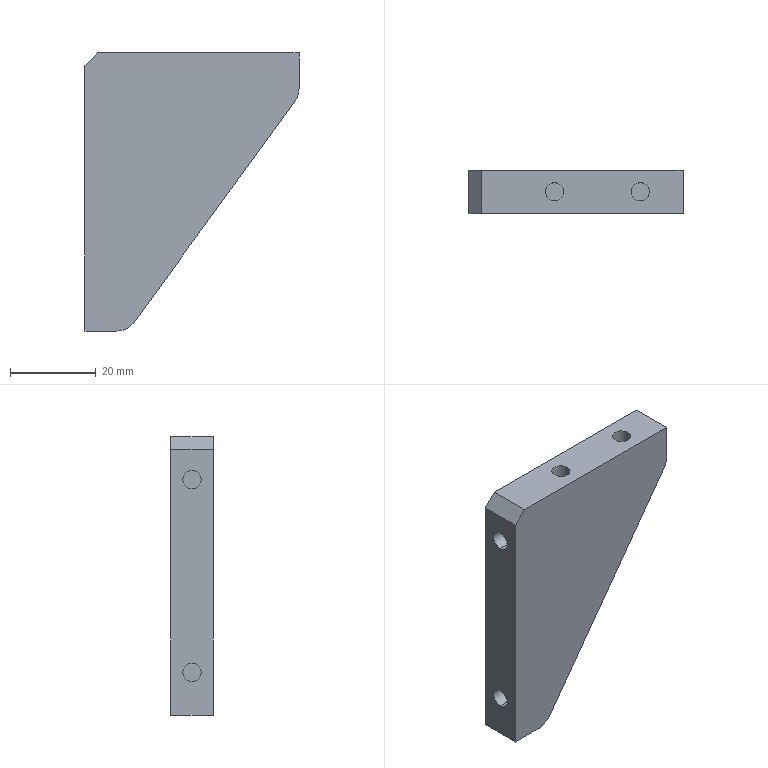Part | STEP file | PN_0009 | 1 solid | 22 faces | box 50 x 10 x 65 mm | volume 20426 mm3 | plane 12 | cylinder 10 | commonest cylinder face diameters 4.3 x8 10 x2
STEP:
#1=CARTESIAN_POINT('',(0.,0.,0.));
#2=DIRECTION('',(0.,0.,1.));
#3=DIRECTION('',(1.,0.,0.));
#4=AXIS2_PLACEMENT_3D('',#1,#2,#3);
#5=CARTESIAN_POINT('',(142.2,-67.,62.));
#6=VERTEX_POINT('',#5);
#7=CARTESIAN_POINT('',(139.2,-67.,59.));
#8=VERTEX_POINT('',#7);
#9=CARTESIAN_POINT('',(142.2,-67.,62.));
#10=DIRECTION('',(-0.7071,0.,-0.7071));
#11=VECTOR('',#10,1.);
#12=LINE('',#9,#11);
#13=CARTESIAN_POINT('',(0.,-67.,0.));
#14=DIRECTION('',(0.,-1.,0.));
#15=DIRECTION('',(1.,0.,0.));
#16=AXIS2_PLACEMENT_3D('',#13,#14,#15);
#17=PLANE('',#16);
#18=CARTESIAN_POINT('',(142.2,62.));
#19=DIRECTION('',(-0.7071,-0.7071));
#20=VECTOR('',#19,1.);
#21=LINE('',#18,#20);
#22=(GEOMETRIC_REPRESENTATION_CONTEXT(2)PARAMETRIC_REPRESENTATION_CONTEXT()REPRESENTATION_CONTEXT('',''));
#23=DEFINITIONAL_REPRESENTATION('',(#21),#22);
#24=PCURVE('',#17,#23);
#25=CARTESIAN_POINT('',(140.7,-62.,60.5));
#26=DIRECTION('',(-0.7071,0.,0.7071));
#27=DIRECTION('',(0.7071,0.,0.7071));
#28=AXIS2_PLACEMENT_3D('',#25,#26,#27);
#29=PLANE('',#28);
#30=CARTESIAN_POINT('',(2.121,-5.));
#31=DIRECTION('',(-1.,0.));
#32=VECTOR('',#31,1.);
#33=LINE('',#30,#32);
#34=(GEOMETRIC_REPRESENTATION_CONTEXT(2)PARAMETRIC_REPRESENTATION_CONTEXT()REPRESENTATION_CONTEXT('',''));
#35=DEFINITIONAL_REPRESENTATION('',(#33),#34);
#36=PCURVE('',#29,#35);
#37=SURFACE_CURVE('',#12,(#24,#36),.PCURVE_S1.);
#38=EDGE_CURVE('',#6,#8,#37,.T.);
#39=ORIENTED_EDGE('',*,*,#38,.F.);
#40=CARTESIAN_POINT('',(189.2,-67.,62.));
#41=VERTEX_POINT('',#40);
#42=CARTESIAN_POINT('',(189.2,-67.,62.));
#43=DIRECTION('',(-1.,0.,0.));
#44=VECTOR('',#43,1.);
#45=LINE('',#42,#44);
#46=CARTESIAN_POINT('',(189.2,62.));
#47=DIRECTION('',(-1.,0.));
#48=VECTOR('',#47,1.);
#49=LINE('',#46,#48);
#50=(GEOMETRIC_REPRESENTATION_CONTEXT(2)PARAMETRIC_REPRESENTATION_CONTEXT()REPRESENTATION_CONTEXT('',''));
#51=DEFINITIONAL_REPRESENTATION('',(#49),#50);
#52=PCURVE('',#17,#51);
#53=CARTESIAN_POINT('',(189.2,-67.,62.));
#54=DIRECTION('',(0.,0.,1.));
#55=DIRECTION('',(-1.,0.,0.));
#56=AXIS2_PLACEMENT_3D('',#53,#54,#55);
#57=PLANE('',#56);
#58=CARTESIAN_POINT('',(0.,0.));
#59=DIRECTION('',(1.,0.));
#60=VECTOR('',#59,1.);
#61=LINE('',#58,#60);
#62=(GEOMETRIC_REPRESENTATION_CONTEXT(2)PARAMETRIC_REPRESENTATION_CONTEXT()REPRESENTATION_CONTEXT('',''));
#63=DEFINITIONAL_REPRESENTATION('',(#61),#62);
#64=PCURVE('',#57,#63);
#65=SURFACE_CURVE('',#45,(#52,#64),.PCURVE_S1.);
#66=EDGE_CURVE('',#41,#6,#65,.T.);
#67=ORIENTED_EDGE('',*,*,#66,.F.);
#68=CARTESIAN_POINT('',(189.2,-67.,53.626));
#69=VERTEX_POINT('',#68);
#70=CARTESIAN_POINT('',(189.2,-67.,53.626));
#71=DIRECTION('',(0.,0.,1.));
#72=VECTOR('',#71,1.);
#73=LINE('',#70,#72);
#74=CARTESIAN_POINT('',(189.2,53.626));
#75=DIRECTION('',(0.,1.));
#76=VECTOR('',#75,1.);
#77=LINE('',#74,#76);
#78=(GEOMETRIC_REPRESENTATION_CONTEXT(2)PARAMETRIC_REPRESENTATION_CONTEXT()REPRESENTATION_CONTEXT('',''));
#79=DEFINITIONAL_REPRESENTATION('',(#77),#78);
#80=PCURVE('',#17,#79);
#81=CARTESIAN_POINT('',(189.2,-67.,52.));
#82=DIRECTION('',(1.,0.,0.));
#83=DIRECTION('',(0.,0.,1.));
#84=AXIS2_PLACEMENT_3D('',#81,#82,#83);
#85=PLANE('',#84);
#86=CARTESIAN_POINT('',(1.626,0.));
#87=DIRECTION('',(1.,0.));
#88=VECTOR('',#87,1.);
#89=LINE('',#86,#88);
#90=(GEOMETRIC_REPRESENTATION_CONTEXT(2)PARAMETRIC_REPRESENTATION_CONTEXT()REPRESENTATION_CONTEXT('',''));
#91=DEFINITIONAL_REPRESENTATION('',(#89),#90);
#92=PCURVE('',#85,#91);
#93=SURFACE_CURVE('',#73,(#80,#92),.PCURVE_S1.);
#94=EDGE_CURVE('',#69,#41,#93,.T.);
#95=ORIENTED_EDGE('',*,*,#94,.F.);
#96=CARTESIAN_POINT('',(188.244,-67.,50.685));
#97=VERTEX_POINT('',#96);
#98=CARTESIAN_POINT('',(184.2,-67.,53.626));
#99=DIRECTION('',(0.,-1.,0.));
#100=DIRECTION('',(0.8087,0.,-0.5882));
#101=AXIS2_PLACEMENT_3D('',#98,#99,#100);
#102=CIRCLE('',#101,5.);
#103=CARTESIAN_POINT('',(184.2,53.626));
#104=DIRECTION('',(0.8087,-0.5882));
#105=AXIS2_PLACEMENT_2D('',#103,#104);
#106=CIRCLE('',#105,5.);
#107=(GEOMETRIC_REPRESENTATION_CONTEXT(2)PARAMETRIC_REPRESENTATION_CONTEXT()REPRESENTATION_CONTEXT('',''));
#108=DEFINITIONAL_REPRESENTATION('',(#106),#107);
#109=PCURVE('',#17,#108);
#110=CARTESIAN_POINT('',(184.2,-67.129,53.626));
#111=DIRECTION('',(0.,1.,0.));
#112=DIRECTION('',(1.,0.,0.));
#113=AXIS2_PLACEMENT_3D('',#110,#111,#112);
#114=CYLINDRICAL_SURFACE('',#113,5.);
#115=CARTESIAN_POINT('',(0.6288,0.1293));
#116=DIRECTION('',(-1.,0.));
#117=VECTOR('',#116,1.);
#118=LINE('',#115,#117);
#119=(GEOMETRIC_REPRESENTATION_CONTEXT(2)PARAMETRIC_REPRESENTATION_CONTEXT()REPRESENTATION_CONTEXT('',''));
#120=DEFINITIONAL_REPRESENTATION('',(#118),#119);
#121=PCURVE('',#114,#120);
#122=SURFACE_CURVE('',#102,(#109,#121),.PCURVE_S1.);
#123=EDGE_CURVE('',#97,#69,#122,.T.);
#124=ORIENTED_EDGE('',*,*,#123,.F.);
#125=CARTESIAN_POINT('',(150.698,-67.,-0.9409));
#126=VERTEX_POINT('',#125);
#127=CARTESIAN_POINT('',(150.698,-67.,-0.9409));
#128=DIRECTION('',(0.5882,0.,0.8087));
#129=VECTOR('',#128,1.);
#130=LINE('',#127,#129);
#131=CARTESIAN_POINT('',(150.698,-0.9409));
#132=DIRECTION('',(0.5882,0.8087));
#133=VECTOR('',#132,1.);
#134=LINE('',#131,#133);
#135=(GEOMETRIC_REPRESENTATION_CONTEXT(2)PARAMETRIC_REPRESENTATION_CONTEXT()REPRESENTATION_CONTEXT('',''));
#136=DEFINITIONAL_REPRESENTATION('',(#134),#135);
#137=PCURVE('',#17,#136);
#138=CARTESIAN_POINT('',(149.2,-67.,-3.));
#139=DIRECTION('',(0.8087,0.,-0.5882));
#140=DIRECTION('',(0.5882,0.,0.8087));
#141=AXIS2_PLACEMENT_3D('',#138,#139,#140);
#142=PLANE('',#141);
#143=CARTESIAN_POINT('',(2.546,0.));
#144=DIRECTION('',(1.,0.));
#145=VECTOR('',#144,1.);
#146=LINE('',#143,#145);
#147=(GEOMETRIC_REPRESENTATION_CONTEXT(2)PARAMETRIC_REPRESENTATION_CONTEXT()REPRESENTATION_CONTEXT('',''));
#148=DEFINITIONAL_REPRESENTATION('',(#146),#147);
#149=PCURVE('',#142,#148);
#150=SURFACE_CURVE('',#130,(#137,#149),.PCURVE_S1.);
#151=EDGE_CURVE('',#126,#97,#150,.T.);
#152=ORIENTED_EDGE('',*,*,#151,.F.);
#153=CARTESIAN_POINT('',(146.654,-67.,-3.));
#154=VERTEX_POINT('',#153);
#155=CARTESIAN_POINT('',(146.654,-67.,2.));
#156=DIRECTION('',(0.,-1.,0.));
#157=DIRECTION('',(0.,0.,-1.));
#158=AXIS2_PLACEMENT_3D('',#155,#156,#157);
#159=CIRCLE('',#158,5.);
#160=CARTESIAN_POINT('',(146.654,2.));
#161=DIRECTION('',(0.,-1.));
#162=AXIS2_PLACEMENT_2D('',#160,#161);
#163=CIRCLE('',#162,5.);
#164=(GEOMETRIC_REPRESENTATION_CONTEXT(2)PARAMETRIC_REPRESENTATION_CONTEXT()REPRESENTATION_CONTEXT('',''));
#165=DEFINITIONAL_REPRESENTATION('',(#163),#164);
#166=PCURVE('',#17,#165);
#167=CARTESIAN_POINT('',(146.654,-67.129,2.));
#168=DIRECTION('',(0.,1.,0.));
#169=DIRECTION('',(0.8087,0.,-0.5882));
#170=AXIS2_PLACEMENT_3D('',#167,#168,#169);
#171=CYLINDRICAL_SURFACE('',#170,5.);
#172=CARTESIAN_POINT('',(0.942,0.1293));
#173=DIRECTION('',(-1.,0.));
#174=VECTOR('',#173,1.);
#175=LINE('',#172,#174);
#176=(GEOMETRIC_REPRESENTATION_CONTEXT(2)PARAMETRIC_REPRESENTATION_CONTEXT()REPRESENTATION_CONTEXT('',''));
#177=DEFINITIONAL_REPRESENTATION('',(#175),#176);
#178=PCURVE('',#171,#177);
#179=SURFACE_CURVE('',#159,(#166,#178),.PCURVE_S1.);
#180=EDGE_CURVE('',#154,#126,#179,.T.);
#181=ORIENTED_EDGE('',*,*,#180,.F.);
#182=CARTESIAN_POINT('',(139.2,-67.,-3.));
#183=VERTEX_POINT('',#182);
#184=CARTESIAN_POINT('',(139.2,-67.,-3.));
#185=DIRECTION('',(1.,0.,0.));
#186=VECTOR('',#185,1.);
#187=LINE('',#184,#186);
#188=CARTESIAN_POINT('',(139.2,-3.));
#189=DIRECTION('',(1.,0.));
#190=VECTOR('',#189,1.);
#191=LINE('',#188,#190);
#192=(GEOMETRIC_REPRESENTATION_CONTEXT(2)PARAMETRIC_REPRESENTATION_CONTEXT()REPRESENTATION_CONTEXT('',''));
#193=DEFINITIONAL_REPRESENTATION('',(#191),#192);
#194=PCURVE('',#17,#193);
#195=CARTESIAN_POINT('',(139.2,-67.,-3.));
#196=DIRECTION('',(0.,0.,-1.));
#197=DIRECTION('',(1.,0.,0.));
#198=AXIS2_PLACEMENT_3D('',#195,#196,#197);
#199=PLANE('',#198);
#200=CARTESIAN_POINT('',(0.,0.));
#201=DIRECTION('',(1.,0.));
#202=VECTOR('',#201,1.);
#203=LINE('',#200,#202);
#204=(GEOMETRIC_REPRESENTATION_CONTEXT(2)PARAMETRIC_REPRESENTATION_CONTEXT()REPRESENTATION_CONTEXT('',''));
#205=DEFINITIONAL_REPRESENTATION('',(#203),#204);
#206=PCURVE('',#199,#205);
#207=SURFACE_CURVE('',#187,(#194,#206),.PCURVE_S1.);
#208=EDGE_CURVE('',#183,#154,#207,.T.);
#209=ORIENTED_EDGE('',*,*,#208,.F.);
#210=CARTESIAN_POINT('',(139.2,-67.,59.));
#211=DIRECTION('',(0.,0.,-1.));
#212=VECTOR('',#211,1.);
#213=LINE('',#210,#212);
#214=CARTESIAN_POINT('',(139.2,59.));
#215=DIRECTION('',(0.,-1.));
#216=VECTOR('',#215,1.);
#217=LINE('',#214,#216);
#218=(GEOMETRIC_REPRESENTATION_CONTEXT(2)PARAMETRIC_REPRESENTATION_CONTEXT()REPRESENTATION_CONTEXT('',''));
#219=DEFINITIONAL_REPRESENTATION('',(#217),#218);
#220=PCURVE('',#17,#219);
#221=CARTESIAN_POINT('',(139.2,-67.,62.));
#222=DIRECTION('',(-1.,0.,0.));
#223=DIRECTION('',(0.,0.,-1.));
#224=AXIS2_PLACEMENT_3D('',#221,#222,#223);
#225=PLANE('',#224);
#226=CARTESIAN_POINT('',(3.,0.));
#227=DIRECTION('',(1.,0.));
#228=VECTOR('',#227,1.);
#229=LINE('',#226,#228);
#230=(GEOMETRIC_REPRESENTATION_CONTEXT(2)PARAMETRIC_REPRESENTATION_CONTEXT()REPRESENTATION_CONTEXT('',''));
#231=DEFINITIONAL_REPRESENTATION('',(#229),#230);
#232=PCURVE('',#225,#231);
#233=SURFACE_CURVE('',#213,(#220,#232),.PCURVE_S1.);
#234=EDGE_CURVE('',#8,#183,#233,.T.);
#235=ORIENTED_EDGE('',*,*,#234,.F.);
#236=EDGE_LOOP('',(#39,#67,#95,#124,#152,#181,#209,#235));
#237=FACE_BOUND('',#236,.F.);
#238=ADVANCED_FACE('',(#237),#17,.T.);
#239=CARTESIAN_POINT('',(139.2,-57.,59.));
#240=VERTEX_POINT('',#239);
#241=CARTESIAN_POINT('',(142.2,-57.,62.));
#242=VERTEX_POINT('',#241);
#243=CARTESIAN_POINT('',(139.2,-57.,59.));
#244=DIRECTION('',(0.7071,0.,0.7071));
#245=VECTOR('',#244,1.);
#246=LINE('',#243,#245);
#247=CARTESIAN_POINT('',(-2.121,5.));
#248=DIRECTION('',(1.,0.));
#249=VECTOR('',#248,1.);
#250=LINE('',#247,#249);
#251=(GEOMETRIC_REPRESENTATION_CONTEXT(2)PARAMETRIC_REPRESENTATION_CONTEXT()REPRESENTATION_CONTEXT('',''));
#252=DEFINITIONAL_REPRESENTATION('',(#250),#251);
#253=PCURVE('',#29,#252);
#254=CARTESIAN_POINT('',(0.,-57.,0.));
#255=DIRECTION('',(0.,-1.,0.));
#256=DIRECTION('',(1.,0.,0.));
#257=AXIS2_PLACEMENT_3D('',#254,#255,#256);
#258=PLANE('',#257);
#259=CARTESIAN_POINT('',(139.2,59.));
#260=DIRECTION('',(0.7071,0.7071));
#261=VECTOR('',#260,1.);
#262=LINE('',#259,#261);
#263=(GEOMETRIC_REPRESENTATION_CONTEXT(2)PARAMETRIC_REPRESENTATION_CONTEXT()REPRESENTATION_CONTEXT('',''));
#264=DEFINITIONAL_REPRESENTATION('',(#262),#263);
#265=PCURVE('',#258,#264);
#266=SURFACE_CURVE('',#246,(#253,#265),.PCURVE_S1.);
#267=EDGE_CURVE('',#240,#242,#266,.T.);
#268=ORIENTED_EDGE('',*,*,#267,.T.);
#269=CARTESIAN_POINT('',(142.2,-67.,62.));
#270=DIRECTION('',(0.,1.,0.));
#271=VECTOR('',#270,1.);
#272=LINE('',#269,#271);
#273=CARTESIAN_POINT('',(2.121,-5.));
#274=DIRECTION('',(0.,1.));
#275=VECTOR('',#274,1.);
#276=LINE('',#273,#275);
#277=(GEOMETRIC_REPRESENTATION_CONTEXT(2)PARAMETRIC_REPRESENTATION_CONTEXT()REPRESENTATION_CONTEXT('',''));
#278=DEFINITIONAL_REPRESENTATION('',(#276),#277);
#279=PCURVE('',#29,#278);
#280=CARTESIAN_POINT('',(47.,0.));
#281=DIRECTION('',(0.,-1.));
#282=VECTOR('',#281,1.);
#283=LINE('',#280,#282);
#284=(GEOMETRIC_REPRESENTATION_CONTEXT(2)PARAMETRIC_REPRESENTATION_CONTEXT()REPRESENTATION_CONTEXT('',''));
#285=DEFINITIONAL_REPRESENTATION('',(#283),#284);
#286=PCURVE('',#57,#285);
#287=SURFACE_CURVE('',#272,(#279,#286),.PCURVE_S1.);
#288=EDGE_CURVE('',#6,#242,#287,.T.);
#289=ORIENTED_EDGE('',*,*,#288,.F.);
#290=ORIENTED_EDGE('',*,*,#38,.T.);
#291=CARTESIAN_POINT('',(139.2,-67.,59.));
#292=DIRECTION('',(0.,1.,0.));
#293=VECTOR('',#292,1.);
#294=LINE('',#291,#293);
#295=CARTESIAN_POINT('',(-2.121,-5.));
#296=DIRECTION('',(0.,1.));
#297=VECTOR('',#296,1.);
#298=LINE('',#295,#297);
#299=(GEOMETRIC_REPRESENTATION_CONTEXT(2)PARAMETRIC_REPRESENTATION_CONTEXT()REPRESENTATION_CONTEXT('',''));
#300=DEFINITIONAL_REPRESENTATION('',(#298),#299);
#301=PCURVE('',#29,#300);
#302=CARTESIAN_POINT('',(3.,0.));
#303=DIRECTION('',(0.,-1.));
#304=VECTOR('',#303,1.);
#305=LINE('',#302,#304);
#306=(GEOMETRIC_REPRESENTATION_CONTEXT(2)PARAMETRIC_REPRESENTATION_CONTEXT()REPRESENTATION_CONTEXT('',''));
#307=DEFINITIONAL_REPRESENTATION('',(#305),#306);
#308=PCURVE('',#225,#307);
#309=SURFACE_CURVE('',#294,(#301,#308),.PCURVE_S1.);
#310=EDGE_CURVE('',#8,#240,#309,.T.);
#311=ORIENTED_EDGE('',*,*,#310,.T.);
#312=EDGE_LOOP('',(#268,#289,#290,#311));
#313=FACE_BOUND('',#312,.F.);
#314=ADVANCED_FACE('',(#313),#29,.T.);
#315=ORIENTED_EDGE('',*,*,#267,.F.);
#316=CARTESIAN_POINT('',(139.2,-57.,-3.));
#317=VERTEX_POINT('',#316);
#318=CARTESIAN_POINT('',(139.2,-57.,59.));
#319=DIRECTION('',(0.,0.,-1.));
#320=VECTOR('',#319,1.);
#321=LINE('',#318,#320);
#322=CARTESIAN_POINT('',(139.2,59.));
#323=DIRECTION('',(0.,-1.));
#324=VECTOR('',#323,1.);
#325=LINE('',#322,#324);
#326=(GEOMETRIC_REPRESENTATION_CONTEXT(2)PARAMETRIC_REPRESENTATION_CONTEXT()REPRESENTATION_CONTEXT('',''));
#327=DEFINITIONAL_REPRESENTATION('',(#325),#326);
#328=PCURVE('',#258,#327);
#329=CARTESIAN_POINT('',(3.,-10.));
#330=DIRECTION('',(1.,0.));
#331=VECTOR('',#330,1.);
#332=LINE('',#329,#331);
#333=(GEOMETRIC_REPRESENTATION_CONTEXT(2)PARAMETRIC_REPRESENTATION_CONTEXT()REPRESENTATION_CONTEXT('',''));
#334=DEFINITIONAL_REPRESENTATION('',(#332),#333);
#335=PCURVE('',#225,#334);
#336=SURFACE_CURVE('',#321,(#328,#335),.PCURVE_S1.);
#337=EDGE_CURVE('',#240,#317,#336,.T.);
#338=ORIENTED_EDGE('',*,*,#337,.T.);
#339=CARTESIAN_POINT('',(146.654,-57.,-3.));
#340=VERTEX_POINT('',#339);
#341=CARTESIAN_POINT('',(139.2,-57.,-3.));
#342=DIRECTION('',(1.,0.,0.));
#343=VECTOR('',#342,1.);
#344=LINE('',#341,#343);
#345=CARTESIAN_POINT('',(139.2,-3.));
#346=DIRECTION('',(1.,0.));
#347=VECTOR('',#346,1.);
#348=LINE('',#345,#347);
#349=(GEOMETRIC_REPRESENTATION_CONTEXT(2)PARAMETRIC_REPRESENTATION_CONTEXT()REPRESENTATION_CONTEXT('',''));
#350=DEFINITIONAL_REPRESENTATION('',(#348),#349);
#351=PCURVE('',#258,#350);
#352=CARTESIAN_POINT('',(0.,-10.));
#353=DIRECTION('',(1.,0.));
#354=VECTOR('',#353,1.);
#355=LINE('',#352,#354);
#356=(GEOMETRIC_REPRESENTATION_CONTEXT(2)PARAMETRIC_REPRESENTATION_CONTEXT()REPRESENTATION_CONTEXT('',''));
#357=DEFINITIONAL_REPRESENTATION('',(#355),#356);
#358=PCURVE('',#199,#357);
#359=SURFACE_CURVE('',#344,(#351,#358),.PCURVE_S1.);
#360=EDGE_CURVE('',#317,#340,#359,.T.);
#361=ORIENTED_EDGE('',*,*,#360,.T.);
#362=CARTESIAN_POINT('',(150.698,-57.,-0.9409));
#363=VERTEX_POINT('',#362);
#364=CARTESIAN_POINT('',(146.654,-57.,2.));
#365=DIRECTION('',(0.,1.,0.));
#366=DIRECTION('',(0.8087,0.,-0.5882));
#367=AXIS2_PLACEMENT_3D('',#364,#365,#366);
#368=CIRCLE('',#367,5.);
#369=CARTESIAN_POINT('',(150.698,-0.9409));
#370=CARTESIAN_POINT('',(145.604,-7.945));
#371=CARTESIAN_POINT('',(142.085,-0.0315));
#372=CARTESIAN_POINT('',(138.567,7.882));
#373=CARTESIAN_POINT('',(147.179,6.972));
#374=CARTESIAN_POINT('',(155.791,6.063));
#375=CARTESIAN_POINT('',(150.698,-0.9409));
#376=(BOUNDED_CURVE()B_SPLINE_CURVE(2,(#369,#370,#371,#372,#373,#374,#375),.UNSPECIFIED.,.T.,.F.)B_SPLINE_CURVE_WITH_KNOTS((1,2,2,2,2,1),(-2.094,0.,2.094,4.189,6.283,8.378),.UNSPECIFIED.)CURVE()GEOMETRIC_REPRESENTATION_ITEM()RATIONAL_B_SPLINE_CURVE((1.,0.5,1.,0.5,1.,0.5,1.))REPRESENTATION_ITEM(''));
#377=(GEOMETRIC_REPRESENTATION_CONTEXT(2)PARAMETRIC_REPRESENTATION_CONTEXT()REPRESENTATION_CONTEXT('',''));
#378=DEFINITIONAL_REPRESENTATION('',(#376),#377);
#379=PCURVE('',#258,#378);
#380=CARTESIAN_POINT('',(0.,10.129));
#381=DIRECTION('',(1.,0.));
#382=VECTOR('',#381,1.);
#383=LINE('',#380,#382);
#384=(GEOMETRIC_REPRESENTATION_CONTEXT(2)PARAMETRIC_REPRESENTATION_CONTEXT()REPRESENTATION_CONTEXT('',''));
#385=DEFINITIONAL_REPRESENTATION('',(#383),#384);
#386=PCURVE('',#171,#385);
#387=SURFACE_CURVE('',#368,(#379,#386),.PCURVE_S1.);
#388=EDGE_CURVE('',#363,#340,#387,.T.);
#389=ORIENTED_EDGE('',*,*,#388,.F.);
#390=CARTESIAN_POINT('',(188.244,-57.,50.685));
#391=VERTEX_POINT('',#390);
#392=CARTESIAN_POINT('',(150.698,-57.,-0.9409));
#393=DIRECTION('',(0.5882,0.,0.8087));
#394=VECTOR('',#393,1.);
#395=LINE('',#392,#394);
#396=CARTESIAN_POINT('',(150.698,-0.9409));
#397=DIRECTION('',(0.5882,0.8087));
#398=VECTOR('',#397,1.);
#399=LINE('',#396,#398);
#400=(GEOMETRIC_REPRESENTATION_CONTEXT(2)PARAMETRIC_REPRESENTATION_CONTEXT()REPRESENTATION_CONTEXT('',''));
#401=DEFINITIONAL_REPRESENTATION('',(#399),#400);
#402=PCURVE('',#258,#401);
#403=CARTESIAN_POINT('',(2.546,-10.));
#404=DIRECTION('',(1.,0.));
#405=VECTOR('',#404,1.);
#406=LINE('',#403,#405);
#407=(GEOMETRIC_REPRESENTATION_CONTEXT(2)PARAMETRIC_REPRESENTATION_CONTEXT()REPRESENTATION_CONTEXT('',''));
#408=DEFINITIONAL_REPRESENTATION('',(#406),#407);
#409=PCURVE('',#142,#408);
#410=SURFACE_CURVE('',#395,(#402,#409),.PCURVE_S1.);
#411=EDGE_CURVE('',#363,#391,#410,.T.);
#412=ORIENTED_EDGE('',*,*,#411,.T.);
#413=CARTESIAN_POINT('',(189.2,-57.,53.626));
#414=VERTEX_POINT('',#413);
#415=CARTESIAN_POINT('',(184.2,-57.,53.626));
#416=DIRECTION('',(0.,1.,0.));
#417=DIRECTION('',(1.,0.,0.));
#418=AXIS2_PLACEMENT_3D('',#415,#416,#417);
#419=CIRCLE('',#418,5.);
#420=CARTESIAN_POINT('',(189.2,53.626));
#421=CARTESIAN_POINT('',(189.2,44.966));
#422=CARTESIAN_POINT('',(181.7,49.296));
#423=CARTESIAN_POINT('',(174.2,53.626));
#424=CARTESIAN_POINT('',(181.7,57.956));
#425=CARTESIAN_POINT('',(189.2,62.286));
#426=CARTESIAN_POINT('',(189.2,53.626));
#427=(BOUNDED_CURVE()B_SPLINE_CURVE(2,(#420,#421,#422,#423,#424,#425,#426),.UNSPECIFIED.,.T.,.F.)B_SPLINE_CURVE_WITH_KNOTS((1,2,2,2,2,1),(-2.094,0.,2.094,4.189,6.283,8.378),.UNSPECIFIED.)CURVE()GEOMETRIC_REPRESENTATION_ITEM()RATIONAL_B_SPLINE_CURVE((1.,0.5,1.,0.5,1.,0.5,1.))REPRESENTATION_ITEM(''));
#428=(GEOMETRIC_REPRESENTATION_CONTEXT(2)PARAMETRIC_REPRESENTATION_CONTEXT()REPRESENTATION_CONTEXT('',''));
#429=DEFINITIONAL_REPRESENTATION('',(#427),#428);
#430=PCURVE('',#258,#429);
#431=CARTESIAN_POINT('',(0.,10.129));
#432=DIRECTION('',(1.,0.));
#433=VECTOR('',#432,1.);
#434=LINE('',#431,#433);
#435=(GEOMETRIC_REPRESENTATION_CONTEXT(2)PARAMETRIC_REPRESENTATION_CONTEXT()REPRESENTATION_CONTEXT('',''));
#436=DEFINITIONAL_REPRESENTATION('',(#434),#435);
#437=PCURVE('',#114,#436);
#438=SURFACE_CURVE('',#419,(#430,#437),.PCURVE_S1.);
#439=EDGE_CURVE('',#414,#391,#438,.T.);
#440=ORIENTED_EDGE('',*,*,#439,.F.);
#441=CARTESIAN_POINT('',(189.2,-57.,62.));
#442=VERTEX_POINT('',#441);
#443=CARTESIAN_POINT('',(189.2,-57.,53.626));
#444=DIRECTION('',(0.,0.,1.));
#445=VECTOR('',#444,1.);
#446=LINE('',#443,#445);
#447=CARTESIAN_POINT('',(189.2,53.626));
#448=DIRECTION('',(0.,1.));
#449=VECTOR('',#448,1.);
#450=LINE('',#447,#449);
#451=(GEOMETRIC_REPRESENTATION_CONTEXT(2)PARAMETRIC_REPRESENTATION_CONTEXT()REPRESENTATION_CONTEXT('',''));
#452=DEFINITIONAL_REPRESENTATION('',(#450),#451);
#453=PCURVE('',#258,#452);
#454=CARTESIAN_POINT('',(1.626,-10.));
#455=DIRECTION('',(1.,0.));
#456=VECTOR('',#455,1.);
#457=LINE('',#454,#456);
#458=(GEOMETRIC_REPRESENTATION_CONTEXT(2)PARAMETRIC_REPRESENTATION_CONTEXT()REPRESENTATION_CONTEXT('',''));
#459=DEFINITIONAL_REPRESENTATION('',(#457),#458);
#460=PCURVE('',#85,#459);
#461=SURFACE_CURVE('',#446,(#453,#460),.PCURVE_S1.);
#462=EDGE_CURVE('',#414,#442,#461,.T.);
#463=ORIENTED_EDGE('',*,*,#462,.T.);
#464=CARTESIAN_POINT('',(189.2,-57.,62.));
#465=DIRECTION('',(-1.,0.,0.));
#466=VECTOR('',#465,1.);
#467=LINE('',#464,#466);
#468=CARTESIAN_POINT('',(189.2,62.));
#469=DIRECTION('',(-1.,0.));
#470=VECTOR('',#469,1.);
#471=LINE('',#468,#470);
#472=(GEOMETRIC_REPRESENTATION_CONTEXT(2)PARAMETRIC_REPRESENTATION_CONTEXT()REPRESENTATION_CONTEXT('',''));
#473=DEFINITIONAL_REPRESENTATION('',(#471),#472);
#474=PCURVE('',#258,#473);
#475=CARTESIAN_POINT('',(0.,-10.));
#476=DIRECTION('',(1.,0.));
#477=VECTOR('',#476,1.);
#478=LINE('',#475,#477);
#479=(GEOMETRIC_REPRESENTATION_CONTEXT(2)PARAMETRIC_REPRESENTATION_CONTEXT()REPRESENTATION_CONTEXT('',''));
#480=DEFINITIONAL_REPRESENTATION('',(#478),#479);
#481=PCURVE('',#57,#480);
#482=SURFACE_CURVE('',#467,(#474,#481),.PCURVE_S1.);
#483=EDGE_CURVE('',#442,#242,#482,.T.);
#484=ORIENTED_EDGE('',*,*,#483,.T.);
#485=EDGE_LOOP('',(#315,#338,#361,#389,#412,#440,#463,#484));
#486=FACE_BOUND('',#485,.F.);
#487=ADVANCED_FACE('',(#486),#258,.F.);
#488=ORIENTED_EDGE('',*,*,#310,.F.);
#489=ORIENTED_EDGE('',*,*,#234,.T.);
#490=CARTESIAN_POINT('',(139.2,-67.,-3.));
#491=DIRECTION('',(0.,1.,0.));
#492=VECTOR('',#491,1.);
#493=LINE('',#490,#492);
#494=CARTESIAN_POINT('',(65.,0.));
#495=DIRECTION('',(0.,-1.));
#496=VECTOR('',#495,1.);
#497=LINE('',#494,#496);
#498=(GEOMETRIC_REPRESENTATION_CONTEXT(2)PARAMETRIC_REPRESENTATION_CONTEXT()REPRESENTATION_CONTEXT('',''));
#499=DEFINITIONAL_REPRESENTATION('',(#497),#498);
#500=PCURVE('',#225,#499);
#501=CARTESIAN_POINT('',(0.,0.));
#502=DIRECTION('',(0.,-1.));
#503=VECTOR('',#502,1.);
#504=LINE('',#501,#503);
#505=(GEOMETRIC_REPRESENTATION_CONTEXT(2)PARAMETRIC_REPRESENTATION_CONTEXT()REPRESENTATION_CONTEXT('',''));
#506=DEFINITIONAL_REPRESENTATION('',(#504),#505);
#507=PCURVE('',#199,#506);
#508=SURFACE_CURVE('',#493,(#500,#507),.PCURVE_S1.);
#509=EDGE_CURVE('',#183,#317,#508,.T.);
#510=ORIENTED_EDGE('',*,*,#509,.T.);
#511=ORIENTED_EDGE('',*,*,#337,.F.);
#512=EDGE_LOOP('',(#488,#489,#510,#511));
#513=FACE_BOUND('',#512,.F.);
#514=CARTESIAN_POINT('',(139.2,-62.,54.15));
#515=VERTEX_POINT('',#514);
#516=CARTESIAN_POINT('',(139.2,-62.,49.85));
#517=VERTEX_POINT('',#516);
#518=CARTESIAN_POINT('',(139.2,-62.,52.));
#519=DIRECTION('',(-1.,0.,0.));
#520=DIRECTION('',(0.,0.,1.));
#521=AXIS2_PLACEMENT_3D('',#518,#519,#520);
#522=CIRCLE('',#521,2.15);
#523=CARTESIAN_POINT('',(10.,-5.));
#524=DIRECTION('',(-1.,0.));
#525=AXIS2_PLACEMENT_2D('',#523,#524);
#526=CIRCLE('',#525,2.15);
#527=(GEOMETRIC_REPRESENTATION_CONTEXT(2)PARAMETRIC_REPRESENTATION_CONTEXT()REPRESENTATION_CONTEXT('',''));
#528=DEFINITIONAL_REPRESENTATION('',(#526),#527);
#529=PCURVE('',#225,#528);
#530=CARTESIAN_POINT('',(139.2,-62.,52.));
#531=DIRECTION('',(-1.,0.,0.));
#532=DIRECTION('',(0.,0.,1.));
#533=AXIS2_PLACEMENT_3D('',#530,#531,#532);
#534=CYLINDRICAL_SURFACE('',#533,2.15);
#535=CARTESIAN_POINT('',(0.,0.));
#536=DIRECTION('',(1.,0.));
#537=VECTOR('',#536,1.);
#538=LINE('',#535,#537);
#539=(GEOMETRIC_REPRESENTATION_CONTEXT(2)PARAMETRIC_REPRESENTATION_CONTEXT()REPRESENTATION_CONTEXT('',''));
#540=DEFINITIONAL_REPRESENTATION('',(#538),#539);
#541=PCURVE('',#534,#540);
#542=SURFACE_CURVE('',#522,(#529,#541),.PCURVE_S1.);
#543=EDGE_CURVE('',#515,#517,#542,.T.);
#544=ORIENTED_EDGE('',*,*,#543,.T.);
#545=CARTESIAN_POINT('',(139.2,-62.,52.));
#546=DIRECTION('',(-1.,0.,0.));
#547=DIRECTION('',(0.,0.,-1.));
#548=AXIS2_PLACEMENT_3D('',#545,#546,#547);
#549=CIRCLE('',#548,2.15);
#550=CARTESIAN_POINT('',(10.,-5.));
#551=DIRECTION('',(1.,0.));
#552=AXIS2_PLACEMENT_2D('',#550,#551);
#553=CIRCLE('',#552,2.15);
#554=(GEOMETRIC_REPRESENTATION_CONTEXT(2)PARAMETRIC_REPRESENTATION_CONTEXT()REPRESENTATION_CONTEXT('',''));
#555=DEFINITIONAL_REPRESENTATION('',(#553),#554);
#556=PCURVE('',#225,#555);
#557=CARTESIAN_POINT('',(139.2,-62.,52.));
#558=DIRECTION('',(-1.,0.,0.));
#559=DIRECTION('',(0.,0.,1.));
#560=AXIS2_PLACEMENT_3D('',#557,#558,#559);
#561=CYLINDRICAL_SURFACE('',#560,2.15);
#562=CARTESIAN_POINT('',(3.142,0.));
#563=DIRECTION('',(1.,0.));
#564=VECTOR('',#563,1.);
#565=LINE('',#562,#564);
#566=(GEOMETRIC_REPRESENTATION_CONTEXT(2)PARAMETRIC_REPRESENTATION_CONTEXT()REPRESENTATION_CONTEXT('',''));
#567=DEFINITIONAL_REPRESENTATION('',(#565),#566);
#568=PCURVE('',#561,#567);
#569=SURFACE_CURVE('',#549,(#556,#568),.PCURVE_S1.);
#570=EDGE_CURVE('',#517,#515,#569,.T.);
#571=ORIENTED_EDGE('',*,*,#570,.T.);
#572=EDGE_LOOP('',(#544,#571));
#573=FACE_BOUND('',#572,.F.);
#574=CARTESIAN_POINT('',(139.2,-62.,9.15));
#575=VERTEX_POINT('',#574);
#576=CARTESIAN_POINT('',(139.2,-62.,4.85));
#577=VERTEX_POINT('',#576);
#578=CARTESIAN_POINT('',(139.2,-62.,7.));
#579=DIRECTION('',(-1.,0.,0.));
#580=DIRECTION('',(0.,0.,1.));
#581=AXIS2_PLACEMENT_3D('',#578,#579,#580);
#582=CIRCLE('',#581,2.15);
#583=CARTESIAN_POINT('',(55.,-5.));
#584=DIRECTION('',(-1.,0.));
#585=AXIS2_PLACEMENT_2D('',#583,#584);
#586=CIRCLE('',#585,2.15);
#587=(GEOMETRIC_REPRESENTATION_CONTEXT(2)PARAMETRIC_REPRESENTATION_CONTEXT()REPRESENTATION_CONTEXT('',''));
#588=DEFINITIONAL_REPRESENTATION('',(#586),#587);
#589=PCURVE('',#225,#588);
#590=CARTESIAN_POINT('',(139.2,-62.,7.));
#591=DIRECTION('',(-1.,0.,0.));
#592=DIRECTION('',(0.,0.,1.));
#593=AXIS2_PLACEMENT_3D('',#590,#591,#592);
#594=CYLINDRICAL_SURFACE('',#593,2.15);
#595=CARTESIAN_POINT('',(0.,0.));
#596=DIRECTION('',(1.,0.));
#597=VECTOR('',#596,1.);
#598=LINE('',#595,#597);
#599=(GEOMETRIC_REPRESENTATION_CONTEXT(2)PARAMETRIC_REPRESENTATION_CONTEXT()REPRESENTATION_CONTEXT('',''));
#600=DEFINITIONAL_REPRESENTATION('',(#598),#599);
#601=PCURVE('',#594,#600);
#602=SURFACE_CURVE('',#582,(#589,#601),.PCURVE_S1.);
#603=EDGE_CURVE('',#575,#577,#602,.T.);
#604=ORIENTED_EDGE('',*,*,#603,.T.);
#605=CARTESIAN_POINT('',(139.2,-62.,7.));
#606=DIRECTION('',(-1.,0.,0.));
#607=DIRECTION('',(0.,0.,-1.));
#608=AXIS2_PLACEMENT_3D('',#605,#606,#607);
#609=CIRCLE('',#608,2.15);
#610=CARTESIAN_POINT('',(55.,-5.));
#611=DIRECTION('',(1.,0.));
#612=AXIS2_PLACEMENT_2D('',#610,#611);
#613=CIRCLE('',#612,2.15);
#614=(GEOMETRIC_REPRESENTATION_CONTEXT(2)PARAMETRIC_REPRESENTATION_CONTEXT()REPRESENTATION_CONTEXT('',''));
#615=DEFINITIONAL_REPRESENTATION('',(#613),#614);
#616=PCURVE('',#225,#615);
#617=CARTESIAN_POINT('',(139.2,-62.,7.));
#618=DIRECTION('',(-1.,0.,0.));
#619=DIRECTION('',(0.,0.,1.));
#620=AXIS2_PLACEMENT_3D('',#617,#618,#619);
#621=CYLINDRICAL_SURFACE('',#620,2.15);
#622=CARTESIAN_POINT('',(3.142,0.));
#623=DIRECTION('',(1.,0.));
#624=VECTOR('',#623,1.);
#625=LINE('',#622,#624);
#626=(GEOMETRIC_REPRESENTATION_CONTEXT(2)PARAMETRIC_REPRESENTATION_CONTEXT()REPRESENTATION_CONTEXT('',''));
#627=DEFINITIONAL_REPRESENTATION('',(#625),#626);
#628=PCURVE('',#621,#627);
#629=SURFACE_CURVE('',#609,(#616,#628),.PCURVE_S1.);
#630=EDGE_CURVE('',#577,#575,#629,.T.);
#631=ORIENTED_EDGE('',*,*,#630,.T.);
#632=EDGE_LOOP('',(#604,#631));
#633=FACE_BOUND('',#632,.F.);
#634=ADVANCED_FACE('',(#513,#573,#633),#225,.T.);
#635=CARTESIAN_POINT('',(146.654,-67.,-3.));
#636=DIRECTION('',(0.,1.,0.));
#637=VECTOR('',#636,1.);
#638=LINE('',#635,#637);
#639=CARTESIAN_POINT('',(7.454,0.));
#640=DIRECTION('',(0.,-1.));
#641=VECTOR('',#640,1.);
#642=LINE('',#639,#641);
#643=(GEOMETRIC_REPRESENTATION_CONTEXT(2)PARAMETRIC_REPRESENTATION_CONTEXT()REPRESENTATION_CONTEXT('',''));
#644=DEFINITIONAL_REPRESENTATION('',(#642),#643);
#645=PCURVE('',#199,#644);
#646=CARTESIAN_POINT('',(0.942,0.1293));
#647=DIRECTION('',(0.,1.));
#648=VECTOR('',#647,1.);
#649=LINE('',#646,#648);
#650=(GEOMETRIC_REPRESENTATION_CONTEXT(2)PARAMETRIC_REPRESENTATION_CONTEXT()REPRESENTATION_CONTEXT('',''));
#651=DEFINITIONAL_REPRESENTATION('',(#649),#650);
#652=PCURVE('',#171,#651);
#653=SURFACE_CURVE('',#638,(#645,#652),.PCURVE_S1.);
#654=EDGE_CURVE('',#154,#340,#653,.T.);
#655=ORIENTED_EDGE('',*,*,#654,.T.);
#656=ORIENTED_EDGE('',*,*,#360,.F.);
#657=ORIENTED_EDGE('',*,*,#509,.F.);
#658=ORIENTED_EDGE('',*,*,#208,.T.);
#659=EDGE_LOOP('',(#655,#656,#657,#658));
#660=FACE_BOUND('',#659,.F.);
#661=ADVANCED_FACE('',(#660),#199,.T.);
#662=CARTESIAN_POINT('',(150.698,-67.,-0.9409));
#663=DIRECTION('',(0.,1.,0.));
#664=VECTOR('',#663,1.);
#665=LINE('',#662,#664);
#666=CARTESIAN_POINT('',(0.,0.1293));
#667=DIRECTION('',(0.,1.));
#668=VECTOR('',#667,1.);
#669=LINE('',#666,#668);
#670=(GEOMETRIC_REPRESENTATION_CONTEXT(2)PARAMETRIC_REPRESENTATION_CONTEXT()REPRESENTATION_CONTEXT('',''));
#671=DEFINITIONAL_REPRESENTATION('',(#669),#670);
#672=PCURVE('',#171,#671);
#673=CARTESIAN_POINT('',(2.546,0.));
#674=DIRECTION('',(0.,-1.));
#675=VECTOR('',#674,1.);
#676=LINE('',#673,#675);
#677=(GEOMETRIC_REPRESENTATION_CONTEXT(2)PARAMETRIC_REPRESENTATION_CONTEXT()REPRESENTATION_CONTEXT('',''));
#678=DEFINITIONAL_REPRESENTATION('',(#676),#677);
#679=PCURVE('',#142,#678);
#680=SURFACE_CURVE('',#665,(#672,#679),.PCURVE_S1.);
#681=EDGE_CURVE('',#126,#363,#680,.T.);
#682=ORIENTED_EDGE('',*,*,#681,.F.);
#683=ORIENTED_EDGE('',*,*,#180,.F.);
#684=ORIENTED_EDGE('',*,*,#654,.T.);
#685=ORIENTED_EDGE('',*,*,#388,.F.);
#686=EDGE_LOOP('',(#682,#683,#684,#685));
#687=FACE_BOUND('',#686,.T.);
#688=ADVANCED_FACE('',(#687),#171,.T.);
#689=CARTESIAN_POINT('',(188.244,-67.,50.685));
#690=DIRECTION('',(0.,1.,0.));
#691=VECTOR('',#690,1.);
#692=LINE('',#689,#691);
#693=CARTESIAN_POINT('',(66.381,0.));
#694=DIRECTION('',(0.,-1.));
#695=VECTOR('',#694,1.);
#696=LINE('',#693,#695);
#697=(GEOMETRIC_REPRESENTATION_CONTEXT(2)PARAMETRIC_REPRESENTATION_CONTEXT()REPRESENTATION_CONTEXT('',''));
#698=DEFINITIONAL_REPRESENTATION('',(#696),#697);
#699=PCURVE('',#142,#698);
#700=CARTESIAN_POINT('',(0.6288,0.1293));
#701=DIRECTION('',(0.,1.));
#702=VECTOR('',#701,1.);
#703=LINE('',#700,#702);
#704=(GEOMETRIC_REPRESENTATION_CONTEXT(2)PARAMETRIC_REPRESENTATION_CONTEXT()REPRESENTATION_CONTEXT('',''));
#705=DEFINITIONAL_REPRESENTATION('',(#703),#704);
#706=PCURVE('',#114,#705);
#707=SURFACE_CURVE('',#692,(#699,#706),.PCURVE_S1.);
#708=EDGE_CURVE('',#97,#391,#707,.T.);
#709=ORIENTED_EDGE('',*,*,#708,.T.);
#710=ORIENTED_EDGE('',*,*,#411,.F.);
#711=ORIENTED_EDGE('',*,*,#681,.F.);
#712=ORIENTED_EDGE('',*,*,#151,.T.);
#713=EDGE_LOOP('',(#709,#710,#711,#712));
#714=FACE_BOUND('',#713,.F.);
#715=ADVANCED_FACE('',(#714),#142,.T.);
#716=CARTESIAN_POINT('',(189.2,-67.,53.626));
#717=DIRECTION('',(0.,1.,0.));
#718=VECTOR('',#717,1.);
#719=LINE('',#716,#718);
#720=CARTESIAN_POINT('',(0.,0.1293));
#721=DIRECTION('',(0.,1.));
#722=VECTOR('',#721,1.);
#723=LINE('',#720,#722);
#724=(GEOMETRIC_REPRESENTATION_CONTEXT(2)PARAMETRIC_REPRESENTATION_CONTEXT()REPRESENTATION_CONTEXT('',''));
#725=DEFINITIONAL_REPRESENTATION('',(#723),#724);
#726=PCURVE('',#114,#725);
#727=CARTESIAN_POINT('',(1.626,0.));
#728=DIRECTION('',(0.,-1.));
#729=VECTOR('',#728,1.);
#730=LINE('',#727,#729);
#731=(GEOMETRIC_REPRESENTATION_CONTEXT(2)PARAMETRIC_REPRESENTATION_CONTEXT()REPRESENTATION_CONTEXT('',''));
#732=DEFINITIONAL_REPRESENTATION('',(#730),#731);
#733=PCURVE('',#85,#732);
#734=SURFACE_CURVE('',#719,(#726,#733),.PCURVE_S1.);
#735=EDGE_CURVE('',#69,#414,#734,.T.);
#736=ORIENTED_EDGE('',*,*,#735,.F.);
#737=ORIENTED_EDGE('',*,*,#123,.F.);
#738=ORIENTED_EDGE('',*,*,#708,.T.);
#739=ORIENTED_EDGE('',*,*,#439,.F.);
#740=EDGE_LOOP('',(#736,#737,#738,#739));
#741=FACE_BOUND('',#740,.T.);
#742=ADVANCED_FACE('',(#741),#114,.T.);
#743=ORIENTED_EDGE('',*,*,#735,.F.);
#744=ORIENTED_EDGE('',*,*,#94,.T.);
#745=CARTESIAN_POINT('',(189.2,-67.,62.));
#746=DIRECTION('',(0.,1.,0.));
#747=VECTOR('',#746,1.);
#748=LINE('',#745,#747);
#749=CARTESIAN_POINT('',(10.,0.));
#750=DIRECTION('',(0.,-1.));
#751=VECTOR('',#750,1.);
#752=LINE('',#749,#751);
#753=(GEOMETRIC_REPRESENTATION_CONTEXT(2)PARAMETRIC_REPRESENTATION_CONTEXT()REPRESENTATION_CONTEXT('',''));
#754=DEFINITIONAL_REPRESENTATION('',(#752),#753);
#755=PCURVE('',#85,#754);
#756=CARTESIAN_POINT('',(0.,0.));
#757=DIRECTION('',(0.,-1.));
#758=VECTOR('',#757,1.);
#759=LINE('',#756,#758);
#760=(GEOMETRIC_REPRESENTATION_CONTEXT(2)PARAMETRIC_REPRESENTATION_CONTEXT()REPRESENTATION_CONTEXT('',''));
#761=DEFINITIONAL_REPRESENTATION('',(#759),#760);
#762=PCURVE('',#57,#761);
#763=SURFACE_CURVE('',#748,(#755,#762),.PCURVE_S1.);
#764=EDGE_CURVE('',#41,#442,#763,.T.);
#765=ORIENTED_EDGE('',*,*,#764,.T.);
#766=ORIENTED_EDGE('',*,*,#462,.F.);
#767=EDGE_LOOP('',(#743,#744,#765,#766));
#768=FACE_BOUND('',#767,.F.);
#769=ADVANCED_FACE('',(#768),#85,.T.);
#770=ORIENTED_EDGE('',*,*,#288,.T.);
#771=ORIENTED_EDGE('',*,*,#483,.F.);
#772=ORIENTED_EDGE('',*,*,#764,.F.);
#773=ORIENTED_EDGE('',*,*,#66,.T.);
#774=EDGE_LOOP('',(#770,#771,#772,#773));
#775=FACE_BOUND('',#774,.F.);
#776=CARTESIAN_POINT('',(161.35,-62.,62.));
#777=VERTEX_POINT('',#776);
#778=CARTESIAN_POINT('',(157.05,-62.,62.));
#779=VERTEX_POINT('',#778);
#780=CARTESIAN_POINT('',(159.2,-62.,62.));
#781=DIRECTION('',(0.,0.,1.));
#782=DIRECTION('',(1.,0.,0.));
#783=AXIS2_PLACEMENT_3D('',#780,#781,#782);
#784=CIRCLE('',#783,2.15);
#785=CARTESIAN_POINT('',(30.,-5.));
#786=DIRECTION('',(-1.,0.));
#787=AXIS2_PLACEMENT_2D('',#785,#786);
#788=CIRCLE('',#787,2.15);
#789=(GEOMETRIC_REPRESENTATION_CONTEXT(2)PARAMETRIC_REPRESENTATION_CONTEXT()REPRESENTATION_CONTEXT('',''));
#790=DEFINITIONAL_REPRESENTATION('',(#788),#789);
#791=PCURVE('',#57,#790);
#792=CARTESIAN_POINT('',(159.2,-62.,62.));
#793=DIRECTION('',(0.,0.,1.));
#794=DIRECTION('',(1.,0.,0.));
#795=AXIS2_PLACEMENT_3D('',#792,#793,#794);
#796=CYLINDRICAL_SURFACE('',#795,2.15);
#797=CARTESIAN_POINT('',(0.,0.));
#798=DIRECTION('',(1.,0.));
#799=VECTOR('',#798,1.);
#800=LINE('',#797,#799);
#801=(GEOMETRIC_REPRESENTATION_CONTEXT(2)PARAMETRIC_REPRESENTATION_CONTEXT()REPRESENTATION_CONTEXT('',''));
#802=DEFINITIONAL_REPRESENTATION('',(#800),#801);
#803=PCURVE('',#796,#802);
#804=SURFACE_CURVE('',#784,(#791,#803),.PCURVE_S1.);
#805=EDGE_CURVE('',#777,#779,#804,.T.);
#806=ORIENTED_EDGE('',*,*,#805,.T.);
#807=CARTESIAN_POINT('',(159.2,-62.,62.));
#808=DIRECTION('',(0.,0.,1.));
#809=DIRECTION('',(-1.,0.,0.));
#810=AXIS2_PLACEMENT_3D('',#807,#808,#809);
#811=CIRCLE('',#810,2.15);
#812=CARTESIAN_POINT('',(30.,-5.));
#813=DIRECTION('',(1.,0.));
#814=AXIS2_PLACEMENT_2D('',#812,#813);
#815=CIRCLE('',#814,2.15);
#816=(GEOMETRIC_REPRESENTATION_CONTEXT(2)PARAMETRIC_REPRESENTATION_CONTEXT()REPRESENTATION_CONTEXT('',''));
#817=DEFINITIONAL_REPRESENTATION('',(#815),#816);
#818=PCURVE('',#57,#817);
#819=CARTESIAN_POINT('',(159.2,-62.,62.));
#820=DIRECTION('',(0.,0.,1.));
#821=DIRECTION('',(1.,0.,0.));
#822=AXIS2_PLACEMENT_3D('',#819,#820,#821);
#823=CYLINDRICAL_SURFACE('',#822,2.15);
#824=CARTESIAN_POINT('',(3.142,0.));
#825=DIRECTION('',(1.,0.));
#826=VECTOR('',#825,1.);
#827=LINE('',#824,#826);
#828=(GEOMETRIC_REPRESENTATION_CONTEXT(2)PARAMETRIC_REPRESENTATION_CONTEXT()REPRESENTATION_CONTEXT('',''));
#829=DEFINITIONAL_REPRESENTATION('',(#827),#828);
#830=PCURVE('',#823,#829);
#831=SURFACE_CURVE('',#811,(#818,#830),.PCURVE_S1.);
#832=EDGE_CURVE('',#779,#777,#831,.T.);
#833=ORIENTED_EDGE('',*,*,#832,.T.);
#834=EDGE_LOOP('',(#806,#833));
#835=FACE_BOUND('',#834,.F.);
#836=CARTESIAN_POINT('',(181.35,-62.,62.));
#837=VERTEX_POINT('',#836);
#838=CARTESIAN_POINT('',(177.05,-62.,62.));
#839=VERTEX_POINT('',#838);
#840=CARTESIAN_POINT('',(179.2,-62.,62.));
#841=DIRECTION('',(0.,0.,1.));
#842=DIRECTION('',(1.,0.,0.));
#843=AXIS2_PLACEMENT_3D('',#840,#841,#842);
#844=CIRCLE('',#843,2.15);
#845=CARTESIAN_POINT('',(10.,-5.));
#846=DIRECTION('',(-1.,0.));
#847=AXIS2_PLACEMENT_2D('',#845,#846);
#848=CIRCLE('',#847,2.15);
#849=(GEOMETRIC_REPRESENTATION_CONTEXT(2)PARAMETRIC_REPRESENTATION_CONTEXT()REPRESENTATION_CONTEXT('',''));
#850=DEFINITIONAL_REPRESENTATION('',(#848),#849);
#851=PCURVE('',#57,#850);
#852=CARTESIAN_POINT('',(179.2,-62.,62.));
#853=DIRECTION('',(0.,0.,1.));
#854=DIRECTION('',(1.,0.,0.));
#855=AXIS2_PLACEMENT_3D('',#852,#853,#854);
#856=CYLINDRICAL_SURFACE('',#855,2.15);
#857=CARTESIAN_POINT('',(0.,0.));
#858=DIRECTION('',(1.,0.));
#859=VECTOR('',#858,1.);
#860=LINE('',#857,#859);
#861=(GEOMETRIC_REPRESENTATION_CONTEXT(2)PARAMETRIC_REPRESENTATION_CONTEXT()REPRESENTATION_CONTEXT('',''));
#862=DEFINITIONAL_REPRESENTATION('',(#860),#861);
#863=PCURVE('',#856,#862);
#864=SURFACE_CURVE('',#844,(#851,#863),.PCURVE_S1.);
#865=EDGE_CURVE('',#837,#839,#864,.T.);
#866=ORIENTED_EDGE('',*,*,#865,.T.);
#867=CARTESIAN_POINT('',(179.2,-62.,62.));
#868=DIRECTION('',(0.,0.,1.));
#869=DIRECTION('',(-1.,0.,0.));
#870=AXIS2_PLACEMENT_3D('',#867,#868,#869);
#871=CIRCLE('',#870,2.15);
#872=CARTESIAN_POINT('',(10.,-5.));
#873=DIRECTION('',(1.,0.));
#874=AXIS2_PLACEMENT_2D('',#872,#873);
#875=CIRCLE('',#874,2.15);
#876=(GEOMETRIC_REPRESENTATION_CONTEXT(2)PARAMETRIC_REPRESENTATION_CONTEXT()REPRESENTATION_CONTEXT('',''));
#877=DEFINITIONAL_REPRESENTATION('',(#875),#876);
#878=PCURVE('',#57,#877);
#879=CARTESIAN_POINT('',(179.2,-62.,62.));
#880=DIRECTION('',(0.,0.,1.));
#881=DIRECTION('',(1.,0.,0.));
#882=AXIS2_PLACEMENT_3D('',#879,#880,#881);
#883=CYLINDRICAL_SURFACE('',#882,2.15);
#884=CARTESIAN_POINT('',(3.142,0.));
#885=DIRECTION('',(1.,0.));
#886=VECTOR('',#885,1.);
#887=LINE('',#884,#886);
#888=(GEOMETRIC_REPRESENTATION_CONTEXT(2)PARAMETRIC_REPRESENTATION_CONTEXT()REPRESENTATION_CONTEXT('',''));
#889=DEFINITIONAL_REPRESENTATION('',(#887),#888);
#890=PCURVE('',#883,#889);
#891=SURFACE_CURVE('',#871,(#878,#890),.PCURVE_S1.);
#892=EDGE_CURVE('',#839,#837,#891,.T.);
#893=ORIENTED_EDGE('',*,*,#892,.T.);
#894=EDGE_LOOP('',(#866,#893));
#895=FACE_BOUND('',#894,.F.);
#896=ADVANCED_FACE('',(#775,#835,#895),#57,.T.);
#897=ORIENTED_EDGE('',*,*,#805,.F.);
#898=CARTESIAN_POINT('',(161.35,-62.,42.));
#899=VERTEX_POINT('',#898);
#900=CARTESIAN_POINT('',(161.35,-62.,62.));
#901=DIRECTION('',(0.,0.,-1.));
#902=VECTOR('',#901,1.);
#903=LINE('',#900,#902);
#904=CARTESIAN_POINT('',(0.,0.));
#905=DIRECTION('',(0.,-1.));
#906=VECTOR('',#905,1.);
#907=LINE('',#904,#906);
#908=(GEOMETRIC_REPRESENTATION_CONTEXT(2)PARAMETRIC_REPRESENTATION_CONTEXT()REPRESENTATION_CONTEXT('',''));
#909=DEFINITIONAL_REPRESENTATION('',(#907),#908);
#910=PCURVE('',#796,#909);
#911=CARTESIAN_POINT('',(6.283,0.));
#912=DIRECTION('',(0.,-1.));
#913=VECTOR('',#912,1.);
#914=LINE('',#911,#913);
#915=(GEOMETRIC_REPRESENTATION_CONTEXT(2)PARAMETRIC_REPRESENTATION_CONTEXT()REPRESENTATION_CONTEXT('',''));
#916=DEFINITIONAL_REPRESENTATION('',(#914),#915);
#917=PCURVE('',#823,#916);
#918=SURFACE_CURVE('',#903,(#910,#917),.PCURVE_S1.);
#919=EDGE_CURVE('',#777,#899,#918,.T.);
#920=ORIENTED_EDGE('',*,*,#919,.T.);
#921=CARTESIAN_POINT('',(157.05,-62.,42.));
#922=VERTEX_POINT('',#921);
#923=CARTESIAN_POINT('',(159.2,-62.,42.));
#924=DIRECTION('',(0.,0.,1.));
#925=DIRECTION('',(1.,0.,0.));
#926=AXIS2_PLACEMENT_3D('',#923,#924,#925);
#927=CIRCLE('',#926,2.15);
#928=CARTESIAN_POINT('',(0.,-20.));
#929=DIRECTION('',(1.,0.));
#930=VECTOR('',#929,1.);
#931=LINE('',#928,#930);
#932=(GEOMETRIC_REPRESENTATION_CONTEXT(2)PARAMETRIC_REPRESENTATION_CONTEXT()REPRESENTATION_CONTEXT('',''));
#933=DEFINITIONAL_REPRESENTATION('',(#931),#932);
#934=PCURVE('',#796,#933);
#935=CARTESIAN_POINT('',(0.,-67.,42.));
#936=DIRECTION('',(0.,0.,1.));
#937=DIRECTION('',(1.,0.,0.));
#938=AXIS2_PLACEMENT_3D('',#935,#936,#937);
#939=PLANE('',#938);
#940=CARTESIAN_POINT('',(159.2,5.));
#941=DIRECTION('',(1.,0.));
#942=AXIS2_PLACEMENT_2D('',#940,#941);
#943=CIRCLE('',#942,2.15);
#944=(GEOMETRIC_REPRESENTATION_CONTEXT(2)PARAMETRIC_REPRESENTATION_CONTEXT()REPRESENTATION_CONTEXT('',''));
#945=DEFINITIONAL_REPRESENTATION('',(#943),#944);
#946=PCURVE('',#939,#945);
#947=SURFACE_CURVE('',#927,(#934,#946),.PCURVE_S1.);
#948=EDGE_CURVE('',#899,#922,#947,.T.);
#949=ORIENTED_EDGE('',*,*,#948,.T.);
#950=CARTESIAN_POINT('',(157.05,-62.,62.));
#951=DIRECTION('',(0.,0.,-1.));
#952=VECTOR('',#951,1.);
#953=LINE('',#950,#952);
#954=CARTESIAN_POINT('',(3.142,0.));
#955=DIRECTION('',(0.,-1.));
#956=VECTOR('',#955,1.);
#957=LINE('',#954,#956);
#958=(GEOMETRIC_REPRESENTATION_CONTEXT(2)PARAMETRIC_REPRESENTATION_CONTEXT()REPRESENTATION_CONTEXT('',''));
#959=DEFINITIONAL_REPRESENTATION('',(#957),#958);
#960=PCURVE('',#796,#959);
#961=CARTESIAN_POINT('',(3.142,0.));
#962=DIRECTION('',(0.,-1.));
#963=VECTOR('',#962,1.);
#964=LINE('',#961,#963);
#965=(GEOMETRIC_REPRESENTATION_CONTEXT(2)PARAMETRIC_REPRESENTATION_CONTEXT()REPRESENTATION_CONTEXT('',''));
#966=DEFINITIONAL_REPRESENTATION('',(#964),#965);
#967=PCURVE('',#823,#966);
#968=SURFACE_CURVE('',#953,(#960,#967),.PCURVE_S1.);
#969=EDGE_CURVE('',#779,#922,#968,.T.);
#970=ORIENTED_EDGE('',*,*,#969,.F.);
#971=EDGE_LOOP('',(#897,#920,#949,#970));
#972=FACE_BOUND('',#971,.F.);
#973=ADVANCED_FACE('',(#972),#796,.F.);
#974=ORIENTED_EDGE('',*,*,#832,.F.);
#975=ORIENTED_EDGE('',*,*,#969,.T.);
#976=CARTESIAN_POINT('',(159.2,-62.,42.));
#977=DIRECTION('',(0.,0.,1.));
#978=DIRECTION('',(-1.,0.,0.));
#979=AXIS2_PLACEMENT_3D('',#976,#977,#978);
#980=CIRCLE('',#979,2.15);
#981=CARTESIAN_POINT('',(3.142,-20.));
#982=DIRECTION('',(1.,0.));
#983=VECTOR('',#982,1.);
#984=LINE('',#981,#983);
#985=(GEOMETRIC_REPRESENTATION_CONTEXT(2)PARAMETRIC_REPRESENTATION_CONTEXT()REPRESENTATION_CONTEXT('',''));
#986=DEFINITIONAL_REPRESENTATION('',(#984),#985);
#987=PCURVE('',#823,#986);
#988=CARTESIAN_POINT('',(159.2,5.));
#989=DIRECTION('',(-1.,0.));
#990=AXIS2_PLACEMENT_2D('',#988,#989);
#991=CIRCLE('',#990,2.15);
#992=(GEOMETRIC_REPRESENTATION_CONTEXT(2)PARAMETRIC_REPRESENTATION_CONTEXT()REPRESENTATION_CONTEXT('',''));
#993=DEFINITIONAL_REPRESENTATION('',(#991),#992);
#994=PCURVE('',#939,#993);
#995=SURFACE_CURVE('',#980,(#987,#994),.PCURVE_S1.);
#996=EDGE_CURVE('',#922,#899,#995,.T.);
#997=ORIENTED_EDGE('',*,*,#996,.T.);
#998=ORIENTED_EDGE('',*,*,#919,.F.);
#999=EDGE_LOOP('',(#974,#975,#997,#998));
#1000=FACE_BOUND('',#999,.F.);
#1001=ADVANCED_FACE('',(#1000),#823,.F.);
#1002=ORIENTED_EDGE('',*,*,#948,.F.);
#1003=ORIENTED_EDGE('',*,*,#996,.F.);
#1004=EDGE_LOOP('',(#1002,#1003));
#1005=FACE_BOUND('',#1004,.F.);
#1006=ADVANCED_FACE('',(#1005),#939,.T.);
#1007=CARTESIAN_POINT('',(181.35,-62.,42.));
#1008=VERTEX_POINT('',#1007);
#1009=CARTESIAN_POINT('',(177.05,-62.,42.));
#1010=VERTEX_POINT('',#1009);
#1011=CARTESIAN_POINT('',(179.2,-62.,42.));
#1012=DIRECTION('',(0.,0.,1.));
#1013=DIRECTION('',(1.,0.,0.));
#1014=AXIS2_PLACEMENT_3D('',#1011,#1012,#1013);
#1015=CIRCLE('',#1014,2.15);
#1016=CARTESIAN_POINT('',(0.,-67.,42.));
#1017=DIRECTION('',(0.,0.,1.));
#1018=DIRECTION('',(1.,0.,0.));
#1019=AXIS2_PLACEMENT_3D('',#1016,#1017,#1018);
#1020=PLANE('',#1019);
#1021=CARTESIAN_POINT('',(179.2,5.));
#1022=DIRECTION('',(1.,0.));
#1023=AXIS2_PLACEMENT_2D('',#1021,#1022);
#1024=CIRCLE('',#1023,2.15);
#1025=(GEOMETRIC_REPRESENTATION_CONTEXT(2)PARAMETRIC_REPRESENTATION_CONTEXT()REPRESENTATION_CONTEXT('',''));
#1026=DEFINITIONAL_REPRESENTATION('',(#1024),#1025);
#1027=PCURVE('',#1020,#1026);
#1028=CARTESIAN_POINT('',(0.,-20.));
#1029=DIRECTION('',(1.,0.));
#1030=VECTOR('',#1029,1.);
#1031=LINE('',#1028,#1030);
#1032=(GEOMETRIC_REPRESENTATION_CONTEXT(2)PARAMETRIC_REPRESENTATION_CONTEXT()REPRESENTATION_CONTEXT('',''));
#1033=DEFINITIONAL_REPRESENTATION('',(#1031),#1032);
#1034=PCURVE('',#856,#1033);
#1035=SURFACE_CURVE('',#1015,(#1027,#1034),.PCURVE_S1.);
#1036=EDGE_CURVE('',#1008,#1010,#1035,.T.);
#1037=ORIENTED_EDGE('',*,*,#1036,.F.);
#1038=CARTESIAN_POINT('',(179.2,-62.,42.));
#1039=DIRECTION('',(0.,0.,1.));
#1040=DIRECTION('',(-1.,0.,0.));
#1041=AXIS2_PLACEMENT_3D('',#1038,#1039,#1040);
#1042=CIRCLE('',#1041,2.15);
#1043=CARTESIAN_POINT('',(179.2,5.));
#1044=DIRECTION('',(-1.,0.));
#1045=AXIS2_PLACEMENT_2D('',#1043,#1044);
#1046=CIRCLE('',#1045,2.15);
#1047=(GEOMETRIC_REPRESENTATION_CONTEXT(2)PARAMETRIC_REPRESENTATION_CONTEXT()REPRESENTATION_CONTEXT('',''));
#1048=DEFINITIONAL_REPRESENTATION('',(#1046),#1047);
#1049=PCURVE('',#1020,#1048);
#1050=CARTESIAN_POINT('',(3.142,-20.));
#1051=DIRECTION('',(1.,0.));
#1052=VECTOR('',#1051,1.);
#1053=LINE('',#1050,#1052);
#1054=(GEOMETRIC_REPRESENTATION_CONTEXT(2)PARAMETRIC_REPRESENTATION_CONTEXT()REPRESENTATION_CONTEXT('',''));
#1055=DEFINITIONAL_REPRESENTATION('',(#1053),#1054);
#1056=PCURVE('',#883,#1055);
#1057=SURFACE_CURVE('',#1042,(#1049,#1056),.PCURVE_S1.);
#1058=EDGE_CURVE('',#1010,#1008,#1057,.T.);
#1059=ORIENTED_EDGE('',*,*,#1058,.F.);
#1060=EDGE_LOOP('',(#1037,#1059));
#1061=FACE_BOUND('',#1060,.F.);
#1062=ADVANCED_FACE('',(#1061),#1020,.T.);
#1063=ORIENTED_EDGE('',*,*,#865,.F.);
#1064=CARTESIAN_POINT('',(181.35,-62.,62.));
#1065=DIRECTION('',(0.,0.,-1.));
#1066=VECTOR('',#1065,1.);
#1067=LINE('',#1064,#1066);
#1068=CARTESIAN_POINT('',(0.,0.));
#1069=DIRECTION('',(0.,-1.));
#1070=VECTOR('',#1069,1.);
#1071=LINE('',#1068,#1070);
#1072=(GEOMETRIC_REPRESENTATION_CONTEXT(2)PARAMETRIC_REPRESENTATION_CONTEXT()REPRESENTATION_CONTEXT('',''));
#1073=DEFINITIONAL_REPRESENTATION('',(#1071),#1072);
#1074=PCURVE('',#856,#1073);
#1075=CARTESIAN_POINT('',(6.283,0.));
#1076=DIRECTION('',(0.,-1.));
#1077=VECTOR('',#1076,1.);
#1078=LINE('',#1075,#1077);
#1079=(GEOMETRIC_REPRESENTATION_CONTEXT(2)PARAMETRIC_REPRESENTATION_CONTEXT()REPRESENTATION_CONTEXT('',''));
#1080=DEFINITIONAL_REPRESENTATION('',(#1078),#1079);
#1081=PCURVE('',#883,#1080);
#1082=SURFACE_CURVE('',#1067,(#1074,#1081),.PCURVE_S1.);
#1083=EDGE_CURVE('',#837,#1008,#1082,.T.);
#1084=ORIENTED_EDGE('',*,*,#1083,.T.);
#1085=ORIENTED_EDGE('',*,*,#1036,.T.);
#1086=CARTESIAN_POINT('',(177.05,-62.,62.));
#1087=DIRECTION('',(0.,0.,-1.));
#1088=VECTOR('',#1087,1.);
#1089=LINE('',#1086,#1088);
#1090=CARTESIAN_POINT('',(3.142,0.));
#1091=DIRECTION('',(0.,-1.));
#1092=VECTOR('',#1091,1.);
#1093=LINE('',#1090,#1092);
#1094=(GEOMETRIC_REPRESENTATION_CONTEXT(2)PARAMETRIC_REPRESENTATION_CONTEXT()REPRESENTATION_CONTEXT('',''));
#1095=DEFINITIONAL_REPRESENTATION('',(#1093),#1094);
#1096=PCURVE('',#856,#1095);
#1097=CARTESIAN_POINT('',(3.142,0.));
#1098=DIRECTION('',(0.,-1.));
#1099=VECTOR('',#1098,1.);
#1100=LINE('',#1097,#1099);
#1101=(GEOMETRIC_REPRESENTATION_CONTEXT(2)PARAMETRIC_REPRESENTATION_CONTEXT()REPRESENTATION_CONTEXT('',''));
#1102=DEFINITIONAL_REPRESENTATION('',(#1100),#1101);
#1103=PCURVE('',#883,#1102);
#1104=SURFACE_CURVE('',#1089,(#1096,#1103),.PCURVE_S1.);
#1105=EDGE_CURVE('',#839,#1010,#1104,.T.);
#1106=ORIENTED_EDGE('',*,*,#1105,.F.);
#1107=EDGE_LOOP('',(#1063,#1084,#1085,#1106));
#1108=FACE_BOUND('',#1107,.F.);
#1109=ADVANCED_FACE('',(#1108),#856,.F.);
#1110=ORIENTED_EDGE('',*,*,#892,.F.);
#1111=ORIENTED_EDGE('',*,*,#1105,.T.);
#1112=ORIENTED_EDGE('',*,*,#1058,.T.);
#1113=ORIENTED_EDGE('',*,*,#1083,.F.);
#1114=EDGE_LOOP('',(#1110,#1111,#1112,#1113));
#1115=FACE_BOUND('',#1114,.F.);
#1116=ADVANCED_FACE('',(#1115),#883,.F.);
#1117=ORIENTED_EDGE('',*,*,#543,.F.);
#1118=CARTESIAN_POINT('',(154.2,-62.,54.15));
#1119=VERTEX_POINT('',#1118);
#1120=CARTESIAN_POINT('',(139.2,-62.,54.15));
#1121=DIRECTION('',(1.,0.,0.));
#1122=VECTOR('',#1121,1.);
#1123=LINE('',#1120,#1122);
#1124=CARTESIAN_POINT('',(0.,0.));
#1125=DIRECTION('',(0.,-1.));
#1126=VECTOR('',#1125,1.);
#1127=LINE('',#1124,#1126);
#1128=(GEOMETRIC_REPRESENTATION_CONTEXT(2)PARAMETRIC_REPRESENTATION_CONTEXT()REPRESENTATION_CONTEXT('',''));
#1129=DEFINITIONAL_REPRESENTATION('',(#1127),#1128);
#1130=PCURVE('',#534,#1129);
#1131=CARTESIAN_POINT('',(6.283,0.));
#1132=DIRECTION('',(0.,-1.));
#1133=VECTOR('',#1132,1.);
#1134=LINE('',#1131,#1133);
#1135=(GEOMETRIC_REPRESENTATION_CONTEXT(2)PARAMETRIC_REPRESENTATION_CONTEXT()REPRESENTATION_CONTEXT('',''));
#1136=DEFINITIONAL_REPRESENTATION('',(#1134),#1135);
#1137=PCURVE('',#561,#1136);
#1138=SURFACE_CURVE('',#1123,(#1130,#1137),.PCURVE_S1.);
#1139=EDGE_CURVE('',#515,#1119,#1138,.T.);
#1140=ORIENTED_EDGE('',*,*,#1139,.T.);
#1141=CARTESIAN_POINT('',(154.2,-62.,49.85));
#1142=VERTEX_POINT('',#1141);
#1143=CARTESIAN_POINT('',(154.2,-62.,52.));
#1144=DIRECTION('',(-1.,0.,0.));
#1145=DIRECTION('',(0.,0.,1.));
#1146=AXIS2_PLACEMENT_3D('',#1143,#1144,#1145);
#1147=CIRCLE('',#1146,2.15);
#1148=CARTESIAN_POINT('',(0.,-15.));
#1149=DIRECTION('',(1.,0.));
#1150=VECTOR('',#1149,1.);
#1151=LINE('',#1148,#1150);
#1152=(GEOMETRIC_REPRESENTATION_CONTEXT(2)PARAMETRIC_REPRESENTATION_CONTEXT()REPRESENTATION_CONTEXT('',''));
#1153=DEFINITIONAL_REPRESENTATION('',(#1151),#1152);
#1154=PCURVE('',#534,#1153);
#1155=CARTESIAN_POINT('',(154.2,-67.,0.));
#1156=DIRECTION('',(-1.,0.,0.));
#1157=DIRECTION('',(0.,0.,1.));
#1158=AXIS2_PLACEMENT_3D('',#1155,#1156,#1157);
#1159=PLANE('',#1158);
#1160=CARTESIAN_POINT('',(52.,5.));
#1161=DIRECTION('',(1.,0.));
#1162=AXIS2_PLACEMENT_2D('',#1160,#1161);
#1163=CIRCLE('',#1162,2.15);
#1164=(GEOMETRIC_REPRESENTATION_CONTEXT(2)PARAMETRIC_REPRESENTATION_CONTEXT()REPRESENTATION_CONTEXT('',''));
#1165=DEFINITIONAL_REPRESENTATION('',(#1163),#1164);
#1166=PCURVE('',#1159,#1165);
#1167=SURFACE_CURVE('',#1147,(#1154,#1166),.PCURVE_S1.);
#1168=EDGE_CURVE('',#1119,#1142,#1167,.T.);
#1169=ORIENTED_EDGE('',*,*,#1168,.T.);
#1170=CARTESIAN_POINT('',(139.2,-62.,49.85));
#1171=DIRECTION('',(1.,0.,0.));
#1172=VECTOR('',#1171,1.);
#1173=LINE('',#1170,#1172);
#1174=CARTESIAN_POINT('',(3.142,0.));
#1175=DIRECTION('',(0.,-1.));
#1176=VECTOR('',#1175,1.);
#1177=LINE('',#1174,#1176);
#1178=(GEOMETRIC_REPRESENTATION_CONTEXT(2)PARAMETRIC_REPRESENTATION_CONTEXT()REPRESENTATION_CONTEXT('',''));
#1179=DEFINITIONAL_REPRESENTATION('',(#1177),#1178);
#1180=PCURVE('',#534,#1179);
#1181=CARTESIAN_POINT('',(3.142,0.));
#1182=DIRECTION('',(0.,-1.));
#1183=VECTOR('',#1182,1.);
#1184=LINE('',#1181,#1183);
#1185=(GEOMETRIC_REPRESENTATION_CONTEXT(2)PARAMETRIC_REPRESENTATION_CONTEXT()REPRESENTATION_CONTEXT('',''));
#1186=DEFINITIONAL_REPRESENTATION('',(#1184),#1185);
#1187=PCURVE('',#561,#1186);
#1188=SURFACE_CURVE('',#1173,(#1180,#1187),.PCURVE_S1.);
#1189=EDGE_CURVE('',#517,#1142,#1188,.T.);
#1190=ORIENTED_EDGE('',*,*,#1189,.F.);
#1191=EDGE_LOOP('',(#1117,#1140,#1169,#1190));
#1192=FACE_BOUND('',#1191,.F.);
#1193=ADVANCED_FACE('',(#1192),#534,.F.);
#1194=ORIENTED_EDGE('',*,*,#570,.F.);
#1195=ORIENTED_EDGE('',*,*,#1189,.T.);
#1196=CARTESIAN_POINT('',(154.2,-62.,52.));
#1197=DIRECTION('',(-1.,0.,0.));
#1198=DIRECTION('',(0.,0.,-1.));
#1199=AXIS2_PLACEMENT_3D('',#1196,#1197,#1198);
#1200=CIRCLE('',#1199,2.15);
#1201=CARTESIAN_POINT('',(3.142,-15.));
#1202=DIRECTION('',(1.,0.));
#1203=VECTOR('',#1202,1.);
#1204=LINE('',#1201,#1203);
#1205=(GEOMETRIC_REPRESENTATION_CONTEXT(2)PARAMETRIC_REPRESENTATION_CONTEXT()REPRESENTATION_CONTEXT('',''));
#1206=DEFINITIONAL_REPRESENTATION('',(#1204),#1205);
#1207=PCURVE('',#561,#1206);
#1208=CARTESIAN_POINT('',(52.,5.));
#1209=DIRECTION('',(-1.,0.));
#1210=AXIS2_PLACEMENT_2D('',#1208,#1209);
#1211=CIRCLE('',#1210,2.15);
#1212=(GEOMETRIC_REPRESENTATION_CONTEXT(2)PARAMETRIC_REPRESENTATION_CONTEXT()REPRESENTATION_CONTEXT('',''));
#1213=DEFINITIONAL_REPRESENTATION('',(#1211),#1212);
#1214=PCURVE('',#1159,#1213);
#1215=SURFACE_CURVE('',#1200,(#1207,#1214),.PCURVE_S1.);
#1216=EDGE_CURVE('',#1142,#1119,#1215,.T.);
#1217=ORIENTED_EDGE('',*,*,#1216,.T.);
#1218=ORIENTED_EDGE('',*,*,#1139,.F.);
#1219=EDGE_LOOP('',(#1194,#1195,#1217,#1218));
#1220=FACE_BOUND('',#1219,.F.);
#1221=ADVANCED_FACE('',(#1220),#561,.F.);
#1222=ORIENTED_EDGE('',*,*,#1168,.F.);
#1223=ORIENTED_EDGE('',*,*,#1216,.F.);
#1224=EDGE_LOOP('',(#1222,#1223));
#1225=FACE_BOUND('',#1224,.F.);
#1226=ADVANCED_FACE('',(#1225),#1159,.T.);
#1227=CARTESIAN_POINT('',(154.2,-62.,9.15));
#1228=VERTEX_POINT('',#1227);
#1229=CARTESIAN_POINT('',(154.2,-62.,4.85));
#1230=VERTEX_POINT('',#1229);
#1231=CARTESIAN_POINT('',(154.2,-62.,7.));
#1232=DIRECTION('',(-1.,0.,0.));
#1233=DIRECTION('',(0.,0.,1.));
#1234=AXIS2_PLACEMENT_3D('',#1231,#1232,#1233);
#1235=CIRCLE('',#1234,2.15);
#1236=CARTESIAN_POINT('',(154.2,-67.,0.));
#1237=DIRECTION('',(-1.,0.,0.));
#1238=DIRECTION('',(0.,0.,1.));
#1239=AXIS2_PLACEMENT_3D('',#1236,#1237,#1238);
#1240=PLANE('',#1239);
#1241=CARTESIAN_POINT('',(7.,5.));
#1242=DIRECTION('',(1.,0.));
#1243=AXIS2_PLACEMENT_2D('',#1241,#1242);
#1244=CIRCLE('',#1243,2.15);
#1245=(GEOMETRIC_REPRESENTATION_CONTEXT(2)PARAMETRIC_REPRESENTATION_CONTEXT()REPRESENTATION_CONTEXT('',''));
#1246=DEFINITIONAL_REPRESENTATION('',(#1244),#1245);
#1247=PCURVE('',#1240,#1246);
#1248=CARTESIAN_POINT('',(0.,-15.));
#1249=DIRECTION('',(1.,0.));
#1250=VECTOR('',#1249,1.);
#1251=LINE('',#1248,#1250);
#1252=(GEOMETRIC_REPRESENTATION_CONTEXT(2)PARAMETRIC_REPRESENTATION_CONTEXT()REPRESENTATION_CONTEXT('',''));
#1253=DEFINITIONAL_REPRESENTATION('',(#1251),#1252);
#1254=PCURVE('',#594,#1253);
#1255=SURFACE_CURVE('',#1235,(#1247,#1254),.PCURVE_S1.);
#1256=EDGE_CURVE('',#1228,#1230,#1255,.T.);
#1257=ORIENTED_EDGE('',*,*,#1256,.F.);
#1258=CARTESIAN_POINT('',(154.2,-62.,7.));
#1259=DIRECTION('',(-1.,0.,0.));
#1260=DIRECTION('',(0.,0.,-1.));
#1261=AXIS2_PLACEMENT_3D('',#1258,#1259,#1260);
#1262=CIRCLE('',#1261,2.15);
#1263=CARTESIAN_POINT('',(7.,5.));
#1264=DIRECTION('',(-1.,0.));
#1265=AXIS2_PLACEMENT_2D('',#1263,#1264);
#1266=CIRCLE('',#1265,2.15);
#1267=(GEOMETRIC_REPRESENTATION_CONTEXT(2)PARAMETRIC_REPRESENTATION_CONTEXT()REPRESENTATION_CONTEXT('',''));
#1268=DEFINITIONAL_REPRESENTATION('',(#1266),#1267);
#1269=PCURVE('',#1240,#1268);
#1270=CARTESIAN_POINT('',(3.142,-15.));
#1271=DIRECTION('',(1.,0.));
#1272=VECTOR('',#1271,1.);
#1273=LINE('',#1270,#1272);
#1274=(GEOMETRIC_REPRESENTATION_CONTEXT(2)PARAMETRIC_REPRESENTATION_CONTEXT()REPRESENTATION_CONTEXT('',''));
#1275=DEFINITIONAL_REPRESENTATION('',(#1273),#1274);
#1276=PCURVE('',#621,#1275);
#1277=SURFACE_CURVE('',#1262,(#1269,#1276),.PCURVE_S1.);
#1278=EDGE_CURVE('',#1230,#1228,#1277,.T.);
#1279=ORIENTED_EDGE('',*,*,#1278,.F.);
#1280=EDGE_LOOP('',(#1257,#1279));
#1281=FACE_BOUND('',#1280,.F.);
#1282=ADVANCED_FACE('',(#1281),#1240,.T.);
#1283=ORIENTED_EDGE('',*,*,#603,.F.);
#1284=CARTESIAN_POINT('',(139.2,-62.,9.15));
#1285=DIRECTION('',(1.,0.,0.));
#1286=VECTOR('',#1285,1.);
#1287=LINE('',#1284,#1286);
#1288=CARTESIAN_POINT('',(0.,0.));
#1289=DIRECTION('',(0.,-1.));
#1290=VECTOR('',#1289,1.);
#1291=LINE('',#1288,#1290);
#1292=(GEOMETRIC_REPRESENTATION_CONTEXT(2)PARAMETRIC_REPRESENTATION_CONTEXT()REPRESENTATION_CONTEXT('',''));
#1293=DEFINITIONAL_REPRESENTATION('',(#1291),#1292);
#1294=PCURVE('',#594,#1293);
#1295=CARTESIAN_POINT('',(6.283,0.));
#1296=DIRECTION('',(0.,-1.));
#1297=VECTOR('',#1296,1.);
#1298=LINE('',#1295,#1297);
#1299=(GEOMETRIC_REPRESENTATION_CONTEXT(2)PARAMETRIC_REPRESENTATION_CONTEXT()REPRESENTATION_CONTEXT('',''));
#1300=DEFINITIONAL_REPRESENTATION('',(#1298),#1299);
#1301=PCURVE('',#621,#1300);
#1302=SURFACE_CURVE('',#1287,(#1294,#1301),.PCURVE_S1.);
#1303=EDGE_CURVE('',#575,#1228,#1302,.T.);
#1304=ORIENTED_EDGE('',*,*,#1303,.T.);
#1305=ORIENTED_EDGE('',*,*,#1256,.T.);
#1306=CARTESIAN_POINT('',(139.2,-62.,4.85));
#1307=DIRECTION('',(1.,0.,0.));
#1308=VECTOR('',#1307,1.);
#1309=LINE('',#1306,#1308);
#1310=CARTESIAN_POINT('',(3.142,0.));
#1311=DIRECTION('',(0.,-1.));
#1312=VECTOR('',#1311,1.);
#1313=LINE('',#1310,#1312);
#1314=(GEOMETRIC_REPRESENTATION_CONTEXT(2)PARAMETRIC_REPRESENTATION_CONTEXT()REPRESENTATION_CONTEXT('',''));
#1315=DEFINITIONAL_REPRESENTATION('',(#1313),#1314);
#1316=PCURVE('',#594,#1315);
#1317=CARTESIAN_POINT('',(3.142,0.));
#1318=DIRECTION('',(0.,-1.));
#1319=VECTOR('',#1318,1.);
#1320=LINE('',#1317,#1319);
#1321=(GEOMETRIC_REPRESENTATION_CONTEXT(2)PARAMETRIC_REPRESENTATION_CONTEXT()REPRESENTATION_CONTEXT('',''));
#1322=DEFINITIONAL_REPRESENTATION('',(#1320),#1321);
#1323=PCURVE('',#621,#1322);
#1324=SURFACE_CURVE('',#1309,(#1316,#1323),.PCURVE_S1.);
#1325=EDGE_CURVE('',#577,#1230,#1324,.T.);
#1326=ORIENTED_EDGE('',*,*,#1325,.F.);
#1327=EDGE_LOOP('',(#1283,#1304,#1305,#1326));
#1328=FACE_BOUND('',#1327,.F.);
#1329=ADVANCED_FACE('',(#1328),#594,.F.);
#1330=ORIENTED_EDGE('',*,*,#630,.F.);
#1331=ORIENTED_EDGE('',*,*,#1325,.T.);
#1332=ORIENTED_EDGE('',*,*,#1278,.T.);
#1333=ORIENTED_EDGE('',*,*,#1303,.F.);
#1334=EDGE_LOOP('',(#1330,#1331,#1332,#1333));
#1335=FACE_BOUND('',#1334,.F.);
#1336=ADVANCED_FACE('',(#1335),#621,.F.);
#1337=CLOSED_SHELL('',(#238,#314,#487,#634,#661,#688,#715,#742,#769,#896,#973,#1001,#1006,#1062,#1109,#1116,#1193,#1221,#1226,#1282,#1329,#1336));
#1338=MANIFOLD_SOLID_BREP('',#1337);
#1339=(LENGTH_UNIT()NAMED_UNIT(*)SI_UNIT(.MILLI.,.METRE.));
#1340=UNCERTAINTY_MEASURE_WITH_UNIT(LENGTH_MEASURE(0.0000001),#1339,'','');
#1341=(NAMED_UNIT(*)PLANE_ANGLE_UNIT()SI_UNIT($,.RADIAN.));
#1342=(NAMED_UNIT(*)SI_UNIT($,.STERADIAN.)SOLID_ANGLE_UNIT());
#1343=(GEOMETRIC_REPRESENTATION_CONTEXT(3)GLOBAL_UNCERTAINTY_ASSIGNED_CONTEXT((#1340))GLOBAL_UNIT_ASSIGNED_CONTEXT((#1339,#1341,#1342))REPRESENTATION_CONTEXT('',''));
#1344=ADVANCED_BREP_SHAPE_REPRESENTATION('',(#4,#1338),#1343);